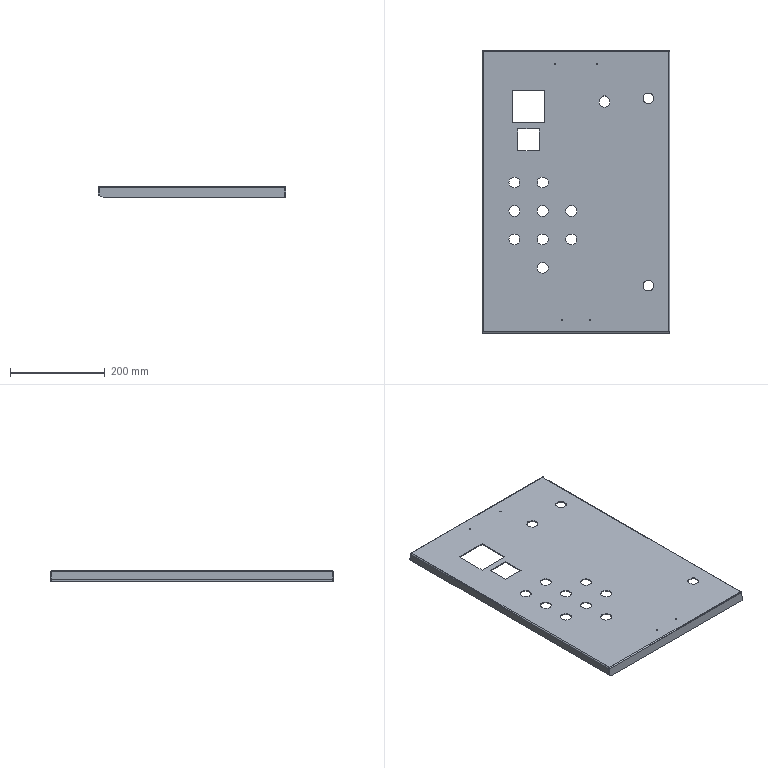Part | SolidWorks | features EdgeFlange 3, Cut 1, FlatPattern 1, SMBaseFlange 1, SheetMetal 1 | 1 solid | 100 faces | box 395 x 595 x 23 mm | volume 521270 mm3 | plane 55 | cylinder 45 | commonest cylinder face diameters 23 x21 2.5 x8 14 x8 0.6 x4 4.6 x4